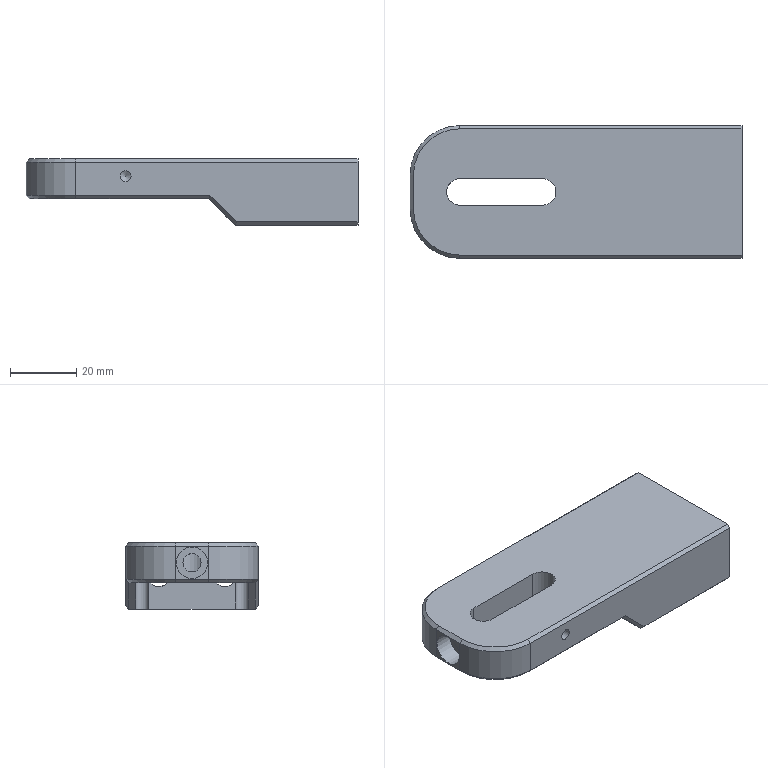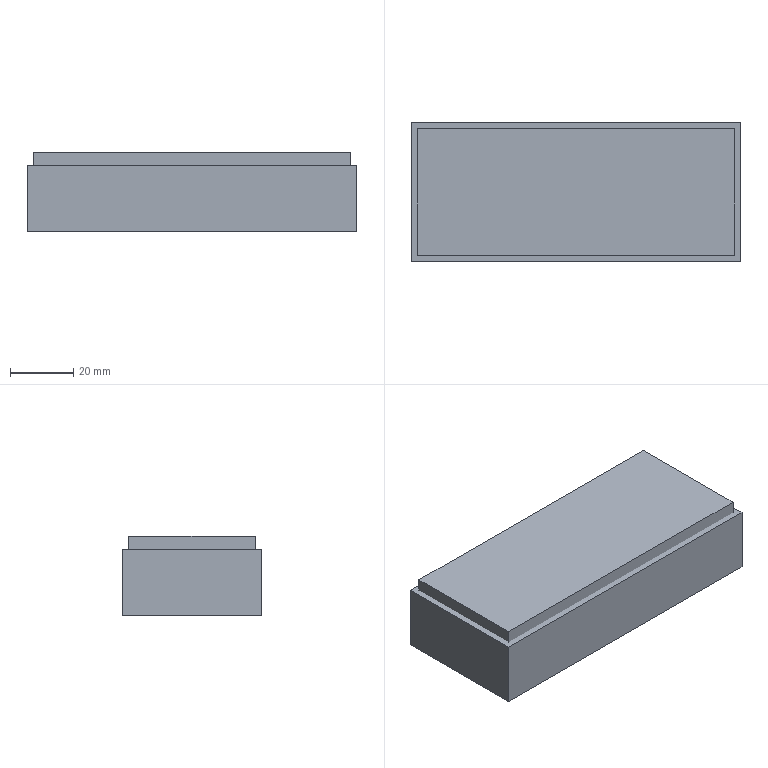CAM job | NX | 3-axis milling | part box 100 x 40 x 20 mm | stock box 104 x 44 x 25 mm
Tools:
number,name,description,diameter,corner_radius,flute_length,length,flutes
1,D63,Milling Tool-5 Parameters,63.0,0.0,50.0,75.0,2
10,D10,Milling Tool-5 Parameters,10.0,0.0,50.0,75.0,2
11,D10JING,Milling Tool-5 Parameters,10.0,0.0,50.0,75.0,2
7,D6A45,Milling Tool-5 Parameters,6.0,0.0,3.0,3.0,2
6,D6,Milling Tool-5 Parameters,6.0,0.0,50.0,75.0,2
4,D4,Milling Tool-5 Parameters,4.0,0.0,50.0,75.0,2
5,D3R0.5,Milling Tool-5 Parameters,3.0,0.5,50.0,75.0,2
Operations:
program,operation,operation_type,tool,method,geometry_group,spindle_rpm,surface_speed,feed_per_tooth,feed_cut,feed_plunge,cut_length_mm,path_length_mm,cut_time_min,machine_time_min
1-103-40-25毛胚-虎钳,FLOOR_WALL,VolumeBased25DMillingOperation,D63,METHOD,A,6500.0,1286.0,0.0962,1250.0,100.0,179.0,233.0,0.1432,0.1486
1-103-40-25毛胚-虎钳,ADAPTIVE_MILLING,CavityMilling,D10,METHOD,A,7000.0,219.0,0.2143,3000.0,1000.0,957.185,1051.185,0.3211,0.3305
1-103-40-25毛胚-虎钳,ZLEVEL_PROFILE_COPY_1_COPY_COPY,ZLevelMilling,D6,METHOD,A,7000.0,131.0,0.1429,2000.0,100.0,1403.873,1472.873,0.7019,0.7088
1-103-40-25毛胚-虎钳,ZLEVEL_PROFILE_COPY_COPY_1,ZLevelMilling,D10JING,METHOD,A,7000.0,219.0,0.0714,1000.0,100.0,310.432,410.432,0.3104,0.3204
1-103-40-25毛胚-虎钳,ZLEVEL_PROFILE_COPY_1_COPY_COPY_COPY_COPY_2_COPY,ZLevelMilling,D6A45,METHOD,A,7000.0,131.0,0.0714,1000.0,1000.0,343.508,556.767,0.3435,0.3648
1-103-40-25毛胚-虎钳,刀补11,ZLevelMilling,D6,METHOD,A,7000.0,219.0,0.0714,1000.0,100.0,60.154,142.154,0.0602,0.0684
2-103-40-25毛胚-虎钳,FLOOR_WALL_COPY,VolumeBased25DMillingOperation,D63,METHOD,B,6500.0,1286.0,0.0962,1250.0,100.0,875.0,1801.001,0.7,0.7926
2-103-40-25毛胚-虎钳,ADAPTIVE_MILLING_COPY,CavityMilling,D10,METHOD,B,7000.0,219.0,0.2143,3000.0,1000.0,10325.619,12360.765,4.254,4.458
2-103-40-25毛胚-虎钳,ZLEVEL_PROFILE_COPY_1,ZLevelMilling,D4,METHOD,B,7000.0,87.0,0.1071,1500.0,1000.0,1102.162,2147.787,0.774,0.8786
2-103-40-25毛胚-虎钳,FLOOR_WALL_1_COPY_1_COPY,VolumeBased25DMillingOperation,D4,METHOD,B,7000.0,87.0,0.0714,1000.0,100.0,299.333,412.876,0.2993,0.3109
2-103-40-25毛胚-虎钳,FLOOR_WALL_1_COPY_1,VolumeBased25DMillingOperation,D4,METHOD,B,7000.0,87.0,0.0714,1000.0,100.0,1888.907,2234.772,1.889,1.931
2-103-40-25毛胚-虎钳,ZLEVEL_PROFILE_COPY_1_COPY_COPY_COPY_COPY_2_COPY_COPY,ZLevelMilling,D6A45,METHOD,B,7000.0,131.0,0.0714,1000.0,1000.0,230.775,366.76,0.2308,0.2444
2-103-40-25毛胚-虎钳,ZLEVEL_PROFILE_COPY_1_COPY_COPY_COPY_COPY_2_COPY_COPY_COPY,ZLevelMilling,D6A45,METHOD,B,7000.0,131.0,0.0714,1000.0,1000.0,220.592,641.92,0.2206,0.2627
2-103-40-25毛胚-虎钳,ZLEVEL_PROFILE_COPY_1_COPY_1_COPY,ZLevelMilling,D3R0.5,METHOD,B,7000.0,65.0,0.2143,3000.0,1000.0,1429.295,1601.353,0.4815,0.4987
2-103-40-25毛胚-虎钳,ZLEVEL_PROFILE_COPY_1_COPY_1_COPY_COPY,ZLevelMilling,D3R0.5,METHOD,B,7000.0,65.0,0.2143,3000.0,1000.0,1974.546,2079.462,0.6621,0.6726